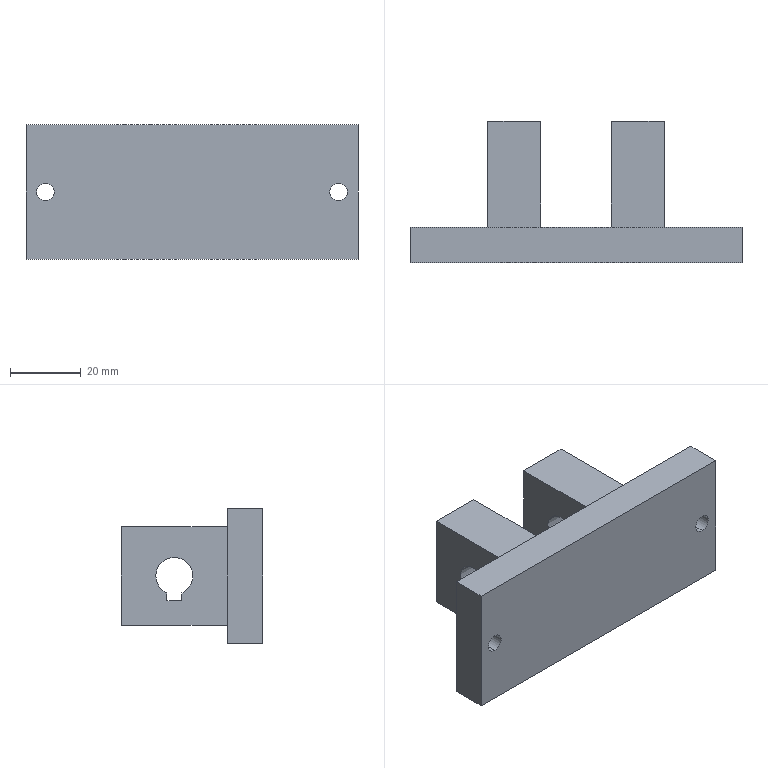Part | SolidWorks | features ICE 5, Extrusion 1, MirrorPattern 1 | 1 solid | 36 faces | box 94 x 40 x 38 mm | volume 57385 mm3 | plane 24 | cylinder 12 | commonest cylinder face diameters 5 x4 8 x4 10.5 x4
STEP:
#1=CARTESIAN_POINT('',(25.,27.1,-4.812));
#2=VERTEX_POINT('',#1);
#3=CARTESIAN_POINT('',(25.,25.,5.25));
#4=VERTEX_POINT('',#3);
#5=CARTESIAN_POINT('',(25.,25.,0.));
#6=DIRECTION('',(1.,0.,0.));
#7=DIRECTION('',(0.,0.,-1.));
#8=AXIS2_PLACEMENT_3D('',#5,#6,#7);
#9=CIRCLE('',#8,5.25);
#10=EDGE_CURVE('',#2,#4,#9,.T.);
#11=ORIENTED_EDGE('',*,*,#10,.T.);
#12=CARTESIAN_POINT('',(10.,25.,5.25));
#13=VERTEX_POINT('',#12);
#14=CARTESIAN_POINT('',(80.,25.,5.25));
#15=DIRECTION('',(-1.,0.,0.));
#16=VECTOR('',#15,1000.);
#17=LINE('',#14,#16);
#18=EDGE_CURVE('',#4,#13,#17,.T.);
#19=ORIENTED_EDGE('',*,*,#18,.T.);
#20=CARTESIAN_POINT('',(10.,27.1,-4.812));
#21=VERTEX_POINT('',#20);
#22=CARTESIAN_POINT('',(10.,25.,0.));
#23=DIRECTION('',(-1.,0.,0.));
#24=DIRECTION('',(0.,0.,1.));
#25=AXIS2_PLACEMENT_3D('',#22,#23,#24);
#26=CIRCLE('',#25,5.25);
#27=EDGE_CURVE('',#13,#21,#26,.T.);
#28=ORIENTED_EDGE('',*,*,#27,.T.);
#29=CARTESIAN_POINT('',(80.,27.1,-4.812));
#30=DIRECTION('',(-1.,0.,0.));
#31=VECTOR('',#30,1000.);
#32=LINE('',#29,#31);
#33=EDGE_CURVE('',#2,#21,#32,.T.);
#34=ORIENTED_EDGE('',*,*,#33,.F.);
#35=EDGE_LOOP('',(#11,#19,#28,#34));
#36=FACE_OUTER_BOUND('',#35,.T.);
#37=CARTESIAN_POINT('',(80.,25.,0.));
#38=DIRECTION('',(-1.,0.,0.));
#39=DIRECTION('',(0.,0.,1.));
#40=AXIS2_PLACEMENT_3D('',#37,#38,#39);
#41=CYLINDRICAL_SURFACE('',#40,5.25);
#42=ADVANCED_FACE('',(#36),#41,.F.);
#43=CARTESIAN_POINT('',(41.5,0.,2.5));
#44=VERTEX_POINT('',#43);
#45=CARTESIAN_POINT('',(41.5,0.,-2.5));
#46=VERTEX_POINT('',#45);
#47=CARTESIAN_POINT('',(41.5,0.,0.));
#48=DIRECTION('',(0.,-1.,0.));
#49=DIRECTION('',(0.,0.,1.));
#50=AXIS2_PLACEMENT_3D('',#47,#48,#49);
#51=CIRCLE('',#50,2.5);
#52=EDGE_CURVE('',#44,#46,#51,.T.);
#53=ORIENTED_EDGE('',*,*,#52,.T.);
#54=CARTESIAN_POINT('',(41.5,5.,-2.5));
#55=VERTEX_POINT('',#54);
#56=CARTESIAN_POINT('',(41.5,0.,-2.5));
#57=DIRECTION('',(0.,1.,0.));
#58=VECTOR('',#57,1000.);
#59=LINE('',#56,#58);
#60=EDGE_CURVE('',#46,#55,#59,.T.);
#61=ORIENTED_EDGE('',*,*,#60,.T.);
#62=CARTESIAN_POINT('',(41.5,5.,2.5));
#63=VERTEX_POINT('',#62);
#64=CARTESIAN_POINT('',(41.5,5.,0.));
#65=DIRECTION('',(0.,-1.,0.));
#66=DIRECTION('',(0.,0.,1.));
#67=AXIS2_PLACEMENT_3D('',#64,#65,#66);
#68=CIRCLE('',#67,2.5);
#69=EDGE_CURVE('',#63,#55,#68,.T.);
#70=ORIENTED_EDGE('',*,*,#69,.F.);
#71=CARTESIAN_POINT('',(41.5,0.,2.5));
#72=DIRECTION('',(0.,1.,0.));
#73=VECTOR('',#72,1000.);
#74=LINE('',#71,#73);
#75=EDGE_CURVE('',#44,#63,#74,.T.);
#76=ORIENTED_EDGE('',*,*,#75,.F.);
#77=EDGE_LOOP('',(#53,#61,#70,#76));
#78=FACE_OUTER_BOUND('',#77,.T.);
#79=CARTESIAN_POINT('',(41.5,0.,0.));
#80=DIRECTION('',(0.,1.,0.));
#81=DIRECTION('',(0.,0.,1.));
#82=AXIS2_PLACEMENT_3D('',#79,#80,#81);
#83=CYLINDRICAL_SURFACE('',#82,2.5);
#84=ADVANCED_FACE('',(#78),#83,.F.);
#85=CARTESIAN_POINT('',(41.5,5.,4.));
#86=VERTEX_POINT('',#85);
#87=CARTESIAN_POINT('',(41.5,5.,-4.));
#88=VERTEX_POINT('',#87);
#89=CARTESIAN_POINT('',(41.5,5.,0.));
#90=DIRECTION('',(0.,-1.,0.));
#91=DIRECTION('',(0.,0.,1.));
#92=AXIS2_PLACEMENT_3D('',#89,#90,#91);
#93=CIRCLE('',#92,4.);
#94=EDGE_CURVE('',#86,#88,#93,.T.);
#95=ORIENTED_EDGE('',*,*,#94,.T.);
#96=CARTESIAN_POINT('',(41.5,10.,-4.));
#97=VERTEX_POINT('',#96);
#98=CARTESIAN_POINT('',(41.5,5.,-4.));
#99=DIRECTION('',(0.,1.,0.));
#100=VECTOR('',#99,1000.);
#101=LINE('',#98,#100);
#102=EDGE_CURVE('',#88,#97,#101,.T.);
#103=ORIENTED_EDGE('',*,*,#102,.T.);
#104=CARTESIAN_POINT('',(41.5,10.,4.));
#105=VERTEX_POINT('',#104);
#106=CARTESIAN_POINT('',(41.5,10.,0.));
#107=DIRECTION('',(0.,-1.,0.));
#108=DIRECTION('',(0.,0.,1.));
#109=AXIS2_PLACEMENT_3D('',#106,#107,#108);
#110=CIRCLE('',#109,4.);
#111=EDGE_CURVE('',#105,#97,#110,.T.);
#112=ORIENTED_EDGE('',*,*,#111,.F.);
#113=CARTESIAN_POINT('',(41.5,5.,4.));
#114=DIRECTION('',(0.,1.,0.));
#115=VECTOR('',#114,1000.);
#116=LINE('',#113,#115);
#117=EDGE_CURVE('',#86,#105,#116,.T.);
#118=ORIENTED_EDGE('',*,*,#117,.F.);
#119=EDGE_LOOP('',(#95,#103,#112,#118));
#120=FACE_OUTER_BOUND('',#119,.T.);
#121=CARTESIAN_POINT('',(41.5,5.,0.));
#122=DIRECTION('',(0.,1.,0.));
#123=DIRECTION('',(0.,0.,1.));
#124=AXIS2_PLACEMENT_3D('',#121,#122,#123);
#125=CYLINDRICAL_SURFACE('',#124,4.);
#126=ADVANCED_FACE('',(#120),#125,.F.);
#127=CARTESIAN_POINT('',(-10.,25.,5.25));
#128=VERTEX_POINT('',#127);
#129=CARTESIAN_POINT('',(-10.,27.1,-4.812));
#130=VERTEX_POINT('',#129);
#131=CARTESIAN_POINT('',(-10.,25.,0.));
#132=DIRECTION('',(-1.,0.,0.));
#133=DIRECTION('',(0.,0.,1.));
#134=AXIS2_PLACEMENT_3D('',#131,#132,#133);
#135=CIRCLE('',#134,5.25);
#136=EDGE_CURVE('',#128,#130,#135,.T.);
#137=ORIENTED_EDGE('',*,*,#136,.F.);
#138=CARTESIAN_POINT('',(-25.,25.,5.25));
#139=VERTEX_POINT('',#138);
#140=CARTESIAN_POINT('',(84.,25.,5.25));
#141=DIRECTION('',(-1.,0.,0.));
#142=VECTOR('',#141,1000.);
#143=LINE('',#140,#142);
#144=EDGE_CURVE('',#128,#139,#143,.T.);
#145=ORIENTED_EDGE('',*,*,#144,.T.);
#146=CARTESIAN_POINT('',(-25.,27.1,-4.812));
#147=VERTEX_POINT('',#146);
#148=CARTESIAN_POINT('',(-25.,25.,0.));
#149=DIRECTION('',(-1.,0.,0.));
#150=DIRECTION('',(0.,0.,1.));
#151=AXIS2_PLACEMENT_3D('',#148,#149,#150);
#152=CIRCLE('',#151,5.25);
#153=EDGE_CURVE('',#139,#147,#152,.T.);
#154=ORIENTED_EDGE('',*,*,#153,.T.);
#155=CARTESIAN_POINT('',(84.,27.1,-4.812));
#156=DIRECTION('',(-1.,0.,0.));
#157=VECTOR('',#156,1000.);
#158=LINE('',#155,#157);
#159=EDGE_CURVE('',#130,#147,#158,.T.);
#160=ORIENTED_EDGE('',*,*,#159,.F.);
#161=EDGE_LOOP('',(#137,#145,#154,#160));
#162=FACE_OUTER_BOUND('',#161,.T.);
#163=CARTESIAN_POINT('',(84.,25.,0.));
#164=DIRECTION('',(-1.,0.,0.));
#165=DIRECTION('',(0.,0.,1.));
#166=AXIS2_PLACEMENT_3D('',#163,#164,#165);
#167=CYLINDRICAL_SURFACE('',#166,5.25);
#168=ADVANCED_FACE('',(#162),#167,.F.);
#169=CARTESIAN_POINT('',(-41.5,0.,-2.5));
#170=VERTEX_POINT('',#169);
#171=CARTESIAN_POINT('',(-41.5,0.,2.5));
#172=VERTEX_POINT('',#171);
#173=CARTESIAN_POINT('',(-41.5,0.,0.));
#174=DIRECTION('',(0.,1.,0.));
#175=DIRECTION('',(0.,0.,1.));
#176=AXIS2_PLACEMENT_3D('',#173,#174,#175);
#177=CIRCLE('',#176,2.5);
#178=EDGE_CURVE('',#170,#172,#177,.T.);
#179=ORIENTED_EDGE('',*,*,#178,.F.);
#180=CARTESIAN_POINT('',(-41.5,5.,-2.5));
#181=VERTEX_POINT('',#180);
#182=CARTESIAN_POINT('',(-41.5,0.,-2.5));
#183=DIRECTION('',(0.,1.,0.));
#184=VECTOR('',#183,1000.);
#185=LINE('',#182,#184);
#186=EDGE_CURVE('',#170,#181,#185,.T.);
#187=ORIENTED_EDGE('',*,*,#186,.T.);
#188=CARTESIAN_POINT('',(-41.5,5.,2.5));
#189=VERTEX_POINT('',#188);
#190=CARTESIAN_POINT('',(-41.5,5.,0.));
#191=DIRECTION('',(0.,1.,0.));
#192=DIRECTION('',(0.,0.,1.));
#193=AXIS2_PLACEMENT_3D('',#190,#191,#192);
#194=CIRCLE('',#193,2.5);
#195=EDGE_CURVE('',#181,#189,#194,.T.);
#196=ORIENTED_EDGE('',*,*,#195,.T.);
#197=CARTESIAN_POINT('',(-41.5,0.,2.5));
#198=DIRECTION('',(0.,1.,0.));
#199=VECTOR('',#198,1000.);
#200=LINE('',#197,#199);
#201=EDGE_CURVE('',#172,#189,#200,.T.);
#202=ORIENTED_EDGE('',*,*,#201,.F.);
#203=EDGE_LOOP('',(#179,#187,#196,#202));
#204=FACE_OUTER_BOUND('',#203,.T.);
#205=CARTESIAN_POINT('',(-41.5,0.,0.));
#206=DIRECTION('',(0.,1.,0.));
#207=DIRECTION('',(0.,0.,1.));
#208=AXIS2_PLACEMENT_3D('',#205,#206,#207);
#209=CYLINDRICAL_SURFACE('',#208,2.5);
#210=ADVANCED_FACE('',(#204),#209,.F.);
#211=CARTESIAN_POINT('',(-41.5,5.,-4.));
#212=VERTEX_POINT('',#211);
#213=CARTESIAN_POINT('',(-41.5,5.,4.));
#214=VERTEX_POINT('',#213);
#215=CARTESIAN_POINT('',(-41.5,5.,0.));
#216=DIRECTION('',(0.,1.,0.));
#217=DIRECTION('',(0.,0.,1.));
#218=AXIS2_PLACEMENT_3D('',#215,#216,#217);
#219=CIRCLE('',#218,4.);
#220=EDGE_CURVE('',#212,#214,#219,.T.);
#221=ORIENTED_EDGE('',*,*,#220,.F.);
#222=CARTESIAN_POINT('',(-41.5,10.,-4.));
#223=VERTEX_POINT('',#222);
#224=CARTESIAN_POINT('',(-41.5,5.,-4.));
#225=DIRECTION('',(0.,1.,0.));
#226=VECTOR('',#225,1000.);
#227=LINE('',#224,#226);
#228=EDGE_CURVE('',#212,#223,#227,.T.);
#229=ORIENTED_EDGE('',*,*,#228,.T.);
#230=CARTESIAN_POINT('',(-41.5,10.,4.));
#231=VERTEX_POINT('',#230);
#232=CARTESIAN_POINT('',(-41.5,10.,0.));
#233=DIRECTION('',(0.,1.,0.));
#234=DIRECTION('',(0.,0.,1.));
#235=AXIS2_PLACEMENT_3D('',#232,#233,#234);
#236=CIRCLE('',#235,4.);
#237=EDGE_CURVE('',#223,#231,#236,.T.);
#238=ORIENTED_EDGE('',*,*,#237,.T.);
#239=CARTESIAN_POINT('',(-41.5,5.,4.));
#240=DIRECTION('',(0.,1.,0.));
#241=VECTOR('',#240,1000.);
#242=LINE('',#239,#241);
#243=EDGE_CURVE('',#214,#231,#242,.T.);
#244=ORIENTED_EDGE('',*,*,#243,.F.);
#245=EDGE_LOOP('',(#221,#229,#238,#244));
#246=FACE_OUTER_BOUND('',#245,.T.);
#247=CARTESIAN_POINT('',(-41.5,5.,0.));
#248=DIRECTION('',(0.,1.,0.));
#249=DIRECTION('',(0.,0.,1.));
#250=AXIS2_PLACEMENT_3D('',#247,#248,#249);
#251=CYLINDRICAL_SURFACE('',#250,4.);
#252=ADVANCED_FACE('',(#246),#251,.F.);
#253=CARTESIAN_POINT('',(-10.,10.,-14.));
#254=VERTEX_POINT('',#253);
#255=CARTESIAN_POINT('',(-10.,10.,14.));
#256=VERTEX_POINT('',#255);
#257=CARTESIAN_POINT('',(-10.,10.,14.));
#258=DIRECTION('',(0.,0.,1.));
#259=VECTOR('',#258,1000.);
#260=LINE('',#257,#259);
#261=EDGE_CURVE('',#254,#256,#260,.T.);
#262=ORIENTED_EDGE('',*,*,#261,.T.);
#263=CARTESIAN_POINT('',(-25.,10.,14.));
#264=VERTEX_POINT('',#263);
#265=CARTESIAN_POINT('',(-10.,10.,14.));
#266=DIRECTION('',(-1.,0.,0.));
#267=VECTOR('',#266,1000.);
#268=LINE('',#265,#267);
#269=EDGE_CURVE('',#256,#264,#268,.T.);
#270=ORIENTED_EDGE('',*,*,#269,.T.);
#271=CARTESIAN_POINT('',(-25.,10.,-14.));
#272=VERTEX_POINT('',#271);
#273=CARTESIAN_POINT('',(-25.,10.,14.));
#274=DIRECTION('',(0.,0.,1.));
#275=VECTOR('',#274,1000.);
#276=LINE('',#273,#275);
#277=EDGE_CURVE('',#272,#264,#276,.T.);
#278=ORIENTED_EDGE('',*,*,#277,.F.);
#279=CARTESIAN_POINT('',(-10.,10.,-14.));
#280=DIRECTION('',(-1.,0.,0.));
#281=VECTOR('',#280,1000.);
#282=LINE('',#279,#281);
#283=EDGE_CURVE('',#254,#272,#282,.T.);
#284=ORIENTED_EDGE('',*,*,#283,.F.);
#285=EDGE_LOOP('',(#262,#270,#278,#284));
#286=FACE_BOUND('',#285,.T.);
#287=CARTESIAN_POINT('',(-41.5,10.,0.));
#288=DIRECTION('',(0.,1.,0.));
#289=DIRECTION('',(0.,0.,1.));
#290=AXIS2_PLACEMENT_3D('',#287,#288,#289);
#291=CIRCLE('',#290,4.);
#292=EDGE_CURVE('',#231,#223,#291,.T.);
#293=ORIENTED_EDGE('',*,*,#292,.F.);
#294=ORIENTED_EDGE('',*,*,#237,.F.);
#295=EDGE_LOOP('',(#293,#294));
#296=FACE_BOUND('',#295,.T.);
#297=CARTESIAN_POINT('',(47.,10.,19.));
#298=VERTEX_POINT('',#297);
#299=CARTESIAN_POINT('',(47.,10.,-19.));
#300=VERTEX_POINT('',#299);
#301=CARTESIAN_POINT('',(47.,10.,19.));
#302=DIRECTION('',(0.,0.,-1.));
#303=VECTOR('',#302,1000.);
#304=LINE('',#301,#303);
#305=EDGE_CURVE('',#298,#300,#304,.T.);
#306=ORIENTED_EDGE('',*,*,#305,.T.);
#307=CARTESIAN_POINT('',(-47.,10.,-19.));
#308=VERTEX_POINT('',#307);
#309=CARTESIAN_POINT('',(-47.,10.,-19.));
#310=DIRECTION('',(-1.,0.,0.));
#311=VECTOR('',#310,1000.);
#312=LINE('',#309,#311);
#313=EDGE_CURVE('',#300,#308,#312,.T.);
#314=ORIENTED_EDGE('',*,*,#313,.T.);
#315=CARTESIAN_POINT('',(-47.,10.,19.));
#316=VERTEX_POINT('',#315);
#317=CARTESIAN_POINT('',(-47.,10.,19.));
#318=DIRECTION('',(0.,0.,1.));
#319=VECTOR('',#318,1000.);
#320=LINE('',#317,#319);
#321=EDGE_CURVE('',#308,#316,#320,.T.);
#322=ORIENTED_EDGE('',*,*,#321,.T.);
#323=CARTESIAN_POINT('',(-47.,10.,19.));
#324=DIRECTION('',(1.,0.,0.));
#325=VECTOR('',#324,1000.);
#326=LINE('',#323,#325);
#327=EDGE_CURVE('',#316,#298,#326,.T.);
#328=ORIENTED_EDGE('',*,*,#327,.T.);
#329=EDGE_LOOP('',(#306,#314,#322,#328));
#330=FACE_OUTER_BOUND('',#329,.T.);
#331=ORIENTED_EDGE('',*,*,#111,.T.);
#332=CARTESIAN_POINT('',(41.5,10.,0.));
#333=DIRECTION('',(0.,-1.,0.));
#334=DIRECTION('',(0.,0.,1.));
#335=AXIS2_PLACEMENT_3D('',#332,#333,#334);
#336=CIRCLE('',#335,4.);
#337=EDGE_CURVE('',#97,#105,#336,.T.);
#338=ORIENTED_EDGE('',*,*,#337,.T.);
#339=EDGE_LOOP('',(#331,#338));
#340=FACE_BOUND('',#339,.T.);
#341=CARTESIAN_POINT('',(10.,10.,-14.));
#342=VERTEX_POINT('',#341);
#343=CARTESIAN_POINT('',(10.,10.,14.));
#344=VERTEX_POINT('',#343);
#345=CARTESIAN_POINT('',(10.,10.,14.));
#346=DIRECTION('',(0.,0.,1.));
#347=VECTOR('',#346,1000.);
#348=LINE('',#345,#347);
#349=EDGE_CURVE('',#342,#344,#348,.T.);
#350=ORIENTED_EDGE('',*,*,#349,.F.);
#351=CARTESIAN_POINT('',(25.,10.,-14.));
#352=VERTEX_POINT('',#351);
#353=CARTESIAN_POINT('',(10.,10.,-14.));
#354=DIRECTION('',(1.,0.,0.));
#355=VECTOR('',#354,1000.);
#356=LINE('',#353,#355);
#357=EDGE_CURVE('',#342,#352,#356,.T.);
#358=ORIENTED_EDGE('',*,*,#357,.T.);
#359=CARTESIAN_POINT('',(25.,10.,14.));
#360=VERTEX_POINT('',#359);
#361=CARTESIAN_POINT('',(25.,10.,14.));
#362=DIRECTION('',(0.,0.,1.));
#363=VECTOR('',#362,1000.);
#364=LINE('',#361,#363);
#365=EDGE_CURVE('',#352,#360,#364,.T.);
#366=ORIENTED_EDGE('',*,*,#365,.T.);
#367=CARTESIAN_POINT('',(10.,10.,14.));
#368=DIRECTION('',(1.,0.,0.));
#369=VECTOR('',#368,1000.);
#370=LINE('',#367,#369);
#371=EDGE_CURVE('',#344,#360,#370,.T.);
#372=ORIENTED_EDGE('',*,*,#371,.F.);
#373=EDGE_LOOP('',(#350,#358,#366,#372));
#374=FACE_BOUND('',#373,.T.);
#375=CARTESIAN_POINT('',(0.,10.,0.));
#376=DIRECTION('',(0.,-1.,0.));
#377=DIRECTION('',(0.,0.,-1.));
#378=AXIS2_PLACEMENT_3D('',#375,#376,#377);
#379=PLANE('',#378);
#380=ADVANCED_FACE('',(#286,#296,#330,#340,#374),#379,.F.);
#381=CARTESIAN_POINT('',(47.,0.,19.));
#382=VERTEX_POINT('',#381);
#383=CARTESIAN_POINT('',(47.,0.,-19.));
#384=VERTEX_POINT('',#383);
#385=CARTESIAN_POINT('',(47.,0.,19.));
#386=DIRECTION('',(0.,0.,-1.));
#387=VECTOR('',#386,1000.);
#388=LINE('',#385,#387);
#389=EDGE_CURVE('',#382,#384,#388,.T.);
#390=ORIENTED_EDGE('',*,*,#389,.T.);
#391=CARTESIAN_POINT('',(47.,10.,-19.));
#392=DIRECTION('',(0.,-1.,0.));
#393=VECTOR('',#392,1000.);
#394=LINE('',#391,#393);
#395=EDGE_CURVE('',#300,#384,#394,.T.);
#396=ORIENTED_EDGE('',*,*,#395,.F.);
#397=ORIENTED_EDGE('',*,*,#305,.F.);
#398=CARTESIAN_POINT('',(47.,10.,19.));
#399=DIRECTION('',(0.,-1.,0.));
#400=VECTOR('',#399,1000.);
#401=LINE('',#398,#400);
#402=EDGE_CURVE('',#298,#382,#401,.T.);
#403=ORIENTED_EDGE('',*,*,#402,.T.);
#404=EDGE_LOOP('',(#390,#396,#397,#403));
#405=FACE_OUTER_BOUND('',#404,.T.);
#406=CARTESIAN_POINT('',(47.,10.,19.));
#407=DIRECTION('',(-1.,0.,0.));
#408=DIRECTION('',(0.,0.,1.));
#409=AXIS2_PLACEMENT_3D('',#406,#407,#408);
#410=PLANE('',#409);
#411=ADVANCED_FACE('',(#405),#410,.F.);
#412=CARTESIAN_POINT('',(-47.,0.,-19.));
#413=VERTEX_POINT('',#412);
#414=CARTESIAN_POINT('',(-47.,0.,-19.));
#415=DIRECTION('',(-1.,0.,0.));
#416=VECTOR('',#415,1000.);
#417=LINE('',#414,#416);
#418=EDGE_CURVE('',#384,#413,#417,.T.);
#419=ORIENTED_EDGE('',*,*,#418,.T.);
#420=CARTESIAN_POINT('',(-47.,10.,-19.));
#421=DIRECTION('',(0.,-1.,0.));
#422=VECTOR('',#421,1000.);
#423=LINE('',#420,#422);
#424=EDGE_CURVE('',#308,#413,#423,.T.);
#425=ORIENTED_EDGE('',*,*,#424,.F.);
#426=ORIENTED_EDGE('',*,*,#313,.F.);
#427=ORIENTED_EDGE('',*,*,#395,.T.);
#428=EDGE_LOOP('',(#419,#425,#426,#427));
#429=FACE_OUTER_BOUND('',#428,.T.);
#430=CARTESIAN_POINT('',(-47.,10.,-19.));
#431=DIRECTION('',(0.,0.,1.));
#432=DIRECTION('',(1.,0.,0.));
#433=AXIS2_PLACEMENT_3D('',#430,#431,#432);
#434=PLANE('',#433);
#435=ADVANCED_FACE('',(#429),#434,.F.);
#436=CARTESIAN_POINT('',(-47.,0.,19.));
#437=VERTEX_POINT('',#436);
#438=CARTESIAN_POINT('',(-47.,0.,19.));
#439=DIRECTION('',(0.,0.,1.));
#440=VECTOR('',#439,1000.);
#441=LINE('',#438,#440);
#442=EDGE_CURVE('',#413,#437,#441,.T.);
#443=ORIENTED_EDGE('',*,*,#442,.T.);
#444=CARTESIAN_POINT('',(-47.,10.,19.));
#445=DIRECTION('',(0.,-1.,0.));
#446=VECTOR('',#445,1000.);
#447=LINE('',#444,#446);
#448=EDGE_CURVE('',#316,#437,#447,.T.);
#449=ORIENTED_EDGE('',*,*,#448,.F.);
#450=ORIENTED_EDGE('',*,*,#321,.F.);
#451=ORIENTED_EDGE('',*,*,#424,.T.);
#452=EDGE_LOOP('',(#443,#449,#450,#451));
#453=FACE_OUTER_BOUND('',#452,.T.);
#454=CARTESIAN_POINT('',(-47.,10.,19.));
#455=DIRECTION('',(1.,0.,0.));
#456=DIRECTION('',(0.,0.,-1.));
#457=AXIS2_PLACEMENT_3D('',#454,#455,#456);
#458=PLANE('',#457);
#459=ADVANCED_FACE('',(#453),#458,.F.);
#460=CARTESIAN_POINT('',(-47.,0.,19.));
#461=DIRECTION('',(1.,0.,0.));
#462=VECTOR('',#461,1000.);
#463=LINE('',#460,#462);
#464=EDGE_CURVE('',#437,#382,#463,.T.);
#465=ORIENTED_EDGE('',*,*,#464,.T.);
#466=ORIENTED_EDGE('',*,*,#402,.F.);
#467=ORIENTED_EDGE('',*,*,#327,.F.);
#468=ORIENTED_EDGE('',*,*,#448,.T.);
#469=EDGE_LOOP('',(#465,#466,#467,#468));
#470=FACE_OUTER_BOUND('',#469,.T.);
#471=CARTESIAN_POINT('',(-47.,10.,19.));
#472=DIRECTION('',(0.,0.,-1.));
#473=DIRECTION('',(-1.,0.,0.));
#474=AXIS2_PLACEMENT_3D('',#471,#472,#473);
#475=PLANE('',#474);
#476=ADVANCED_FACE('',(#470),#475,.F.);
#477=ORIENTED_EDGE('',*,*,#52,.F.);
#478=CARTESIAN_POINT('',(41.5,0.,0.));
#479=DIRECTION('',(0.,-1.,0.));
#480=DIRECTION('',(0.,0.,1.));
#481=AXIS2_PLACEMENT_3D('',#478,#479,#480);
#482=CIRCLE('',#481,2.5);
#483=EDGE_CURVE('',#46,#44,#482,.T.);
#484=ORIENTED_EDGE('',*,*,#483,.F.);
#485=EDGE_LOOP('',(#477,#484));
#486=FACE_BOUND('',#485,.T.);
#487=CARTESIAN_POINT('',(-41.5,0.,0.));
#488=DIRECTION('',(0.,1.,0.));
#489=DIRECTION('',(0.,0.,1.));
#490=AXIS2_PLACEMENT_3D('',#487,#488,#489);
#491=CIRCLE('',#490,2.5);
#492=EDGE_CURVE('',#172,#170,#491,.T.);
#493=ORIENTED_EDGE('',*,*,#492,.T.);
#494=ORIENTED_EDGE('',*,*,#178,.T.);
#495=EDGE_LOOP('',(#493,#494));
#496=FACE_BOUND('',#495,.T.);
#497=ORIENTED_EDGE('',*,*,#389,.F.);
#498=ORIENTED_EDGE('',*,*,#464,.F.);
#499=ORIENTED_EDGE('',*,*,#442,.F.);
#500=ORIENTED_EDGE('',*,*,#418,.F.);
#501=EDGE_LOOP('',(#497,#498,#499,#500));
#502=FACE_OUTER_BOUND('',#501,.T.);
#503=CARTESIAN_POINT('',(0.,0.,0.));
#504=DIRECTION('',(0.,-1.,0.));
#505=DIRECTION('',(0.,0.,-1.));
#506=AXIS2_PLACEMENT_3D('',#503,#504,#505);
#507=PLANE('',#506);
#508=ADVANCED_FACE('',(#486,#496,#502),#507,.T.);
#509=ORIENTED_EDGE('',*,*,#228,.F.);
#510=CARTESIAN_POINT('',(-41.5,5.,0.));
#511=DIRECTION('',(0.,1.,0.));
#512=DIRECTION('',(0.,0.,1.));
#513=AXIS2_PLACEMENT_3D('',#510,#511,#512);
#514=CIRCLE('',#513,4.);
#515=EDGE_CURVE('',#214,#212,#514,.T.);
#516=ORIENTED_EDGE('',*,*,#515,.F.);
#517=ORIENTED_EDGE('',*,*,#243,.T.);
#518=ORIENTED_EDGE('',*,*,#292,.T.);
#519=EDGE_LOOP('',(#509,#516,#517,#518));
#520=FACE_OUTER_BOUND('',#519,.T.);
#521=CARTESIAN_POINT('',(-41.5,5.,0.));
#522=DIRECTION('',(0.,1.,0.));
#523=DIRECTION('',(0.,0.,1.));
#524=AXIS2_PLACEMENT_3D('',#521,#522,#523);
#525=CYLINDRICAL_SURFACE('',#524,4.);
#526=ADVANCED_FACE('',(#520),#525,.F.);
#527=CARTESIAN_POINT('',(-41.5,5.,0.));
#528=DIRECTION('',(0.,1.,0.));
#529=DIRECTION('',(0.,0.,1.));
#530=AXIS2_PLACEMENT_3D('',#527,#528,#529);
#531=CIRCLE('',#530,2.5);
#532=EDGE_CURVE('',#189,#181,#531,.T.);
#533=ORIENTED_EDGE('',*,*,#532,.F.);
#534=ORIENTED_EDGE('',*,*,#195,.F.);
#535=EDGE_LOOP('',(#533,#534));
#536=FACE_BOUND('',#535,.T.);
#537=ORIENTED_EDGE('',*,*,#515,.T.);
#538=ORIENTED_EDGE('',*,*,#220,.T.);
#539=EDGE_LOOP('',(#537,#538));
#540=FACE_OUTER_BOUND('',#539,.T.);
#541=CARTESIAN_POINT('',(-41.5,5.,0.));
#542=DIRECTION('',(0.,1.,0.));
#543=DIRECTION('',(0.,0.,1.));
#544=AXIS2_PLACEMENT_3D('',#541,#542,#543);
#545=PLANE('',#544);
#546=ADVANCED_FACE('',(#536,#540),#545,.T.);
#547=ORIENTED_EDGE('',*,*,#186,.F.);
#548=ORIENTED_EDGE('',*,*,#492,.F.);
#549=ORIENTED_EDGE('',*,*,#201,.T.);
#550=ORIENTED_EDGE('',*,*,#532,.T.);
#551=EDGE_LOOP('',(#547,#548,#549,#550));
#552=FACE_OUTER_BOUND('',#551,.T.);
#553=CARTESIAN_POINT('',(-41.5,0.,0.));
#554=DIRECTION('',(0.,1.,0.));
#555=DIRECTION('',(0.,0.,1.));
#556=AXIS2_PLACEMENT_3D('',#553,#554,#555);
#557=CYLINDRICAL_SURFACE('',#556,2.5);
#558=ADVANCED_FACE('',(#552),#557,.F.);
#559=CARTESIAN_POINT('',(-25.,40.,14.));
#560=VERTEX_POINT('',#559);
#561=CARTESIAN_POINT('',(-25.,10.,14.));
#562=DIRECTION('',(0.,1.,0.));
#563=VECTOR('',#562,1000.);
#564=LINE('',#561,#563);
#565=EDGE_CURVE('',#264,#560,#564,.T.);
#566=ORIENTED_EDGE('',*,*,#565,.F.);
#567=ORIENTED_EDGE('',*,*,#269,.F.);
#568=CARTESIAN_POINT('',(-10.,40.,14.));
#569=VERTEX_POINT('',#568);
#570=CARTESIAN_POINT('',(-10.,10.,14.));
#571=DIRECTION('',(0.,1.,0.));
#572=VECTOR('',#571,1000.);
#573=LINE('',#570,#572);
#574=EDGE_CURVE('',#256,#569,#573,.T.);
#575=ORIENTED_EDGE('',*,*,#574,.T.);
#576=CARTESIAN_POINT('',(-10.,40.,14.));
#577=DIRECTION('',(-1.,0.,0.));
#578=VECTOR('',#577,1000.);
#579=LINE('',#576,#578);
#580=EDGE_CURVE('',#569,#560,#579,.T.);
#581=ORIENTED_EDGE('',*,*,#580,.T.);
#582=EDGE_LOOP('',(#566,#567,#575,#581));
#583=FACE_OUTER_BOUND('',#582,.T.);
#584=CARTESIAN_POINT('',(-10.,10.,14.));
#585=DIRECTION('',(0.,0.,1.));
#586=DIRECTION('',(0.,-1.,0.));
#587=AXIS2_PLACEMENT_3D('',#584,#585,#586);
#588=PLANE('',#587);
#589=ADVANCED_FACE('',(#583),#588,.T.);
#590=CARTESIAN_POINT('',(-25.,40.,-14.));
#591=VERTEX_POINT('',#590);
#592=CARTESIAN_POINT('',(-25.,10.,-14.));
#593=DIRECTION('',(0.,-1.,0.));
#594=VECTOR('',#593,1000.);
#595=LINE('',#592,#594);
#596=EDGE_CURVE('',#591,#272,#595,.T.);
#597=ORIENTED_EDGE('',*,*,#596,.F.);
#598=CARTESIAN_POINT('',(-10.,40.,-14.));
#599=VERTEX_POINT('',#598);
#600=CARTESIAN_POINT('',(-10.,40.,-14.));
#601=DIRECTION('',(-1.,0.,0.));
#602=VECTOR('',#601,1000.);
#603=LINE('',#600,#602);
#604=EDGE_CURVE('',#599,#591,#603,.T.);
#605=ORIENTED_EDGE('',*,*,#604,.F.);
#606=CARTESIAN_POINT('',(-10.,10.,-14.));
#607=DIRECTION('',(0.,-1.,0.));
#608=VECTOR('',#607,1000.);
#609=LINE('',#606,#608);
#610=EDGE_CURVE('',#599,#254,#609,.T.);
#611=ORIENTED_EDGE('',*,*,#610,.T.);
#612=ORIENTED_EDGE('',*,*,#283,.T.);
#613=EDGE_LOOP('',(#597,#605,#611,#612));
#614=FACE_OUTER_BOUND('',#613,.T.);
#615=CARTESIAN_POINT('',(-10.,10.,-14.));
#616=DIRECTION('',(0.,0.,-1.));
#617=DIRECTION('',(-1.,0.,0.));
#618=AXIS2_PLACEMENT_3D('',#615,#616,#617);
#619=PLANE('',#618);
#620=ADVANCED_FACE('',(#614),#619,.T.);
#621=CARTESIAN_POINT('',(-25.,40.,14.));
#622=DIRECTION('',(0.,0.,-1.));
#623=VECTOR('',#622,1000.);
#624=LINE('',#621,#623);
#625=EDGE_CURVE('',#560,#591,#624,.T.);
#626=ORIENTED_EDGE('',*,*,#625,.F.);
#627=ORIENTED_EDGE('',*,*,#580,.F.);
#628=CARTESIAN_POINT('',(-10.,40.,14.));
#629=DIRECTION('',(0.,0.,-1.));
#630=VECTOR('',#629,1000.);
#631=LINE('',#628,#630);
#632=EDGE_CURVE('',#569,#599,#631,.T.);
#633=ORIENTED_EDGE('',*,*,#632,.T.);
#634=ORIENTED_EDGE('',*,*,#604,.T.);
#635=EDGE_LOOP('',(#626,#627,#633,#634));
#636=FACE_OUTER_BOUND('',#635,.T.);
#637=CARTESIAN_POINT('',(-10.,40.,14.));
#638=DIRECTION('',(0.,1.,0.));
#639=DIRECTION('',(0.,0.,1.));
#640=AXIS2_PLACEMENT_3D('',#637,#638,#639);
#641=PLANE('',#640);
#642=ADVANCED_FACE('',(#636),#641,.T.);
#643=CARTESIAN_POINT('',(-10.,27.1,-7.));
#644=VERTEX_POINT('',#643);
#645=CARTESIAN_POINT('',(-10.,27.1,0.));
#646=DIRECTION('',(0.,0.,1.));
#647=VECTOR('',#646,1000.);
#648=LINE('',#645,#647);
#649=EDGE_CURVE('',#644,#130,#648,.T.);
#650=ORIENTED_EDGE('',*,*,#649,.F.);
#651=CARTESIAN_POINT('',(-10.,22.9,-7.));
#652=VERTEX_POINT('',#651);
#653=CARTESIAN_POINT('',(-10.,0.,-7.));
#654=DIRECTION('',(0.,-1.,0.));
#655=VECTOR('',#654,1000.);
#656=LINE('',#653,#655);
#657=EDGE_CURVE('',#644,#652,#656,.T.);
#658=ORIENTED_EDGE('',*,*,#657,.T.);
#659=CARTESIAN_POINT('',(-10.,22.9,-4.812));
#660=VERTEX_POINT('',#659);
#661=CARTESIAN_POINT('',(-10.,22.9,0.));
#662=DIRECTION('',(0.,0.,1.));
#663=VECTOR('',#662,1000.);
#664=LINE('',#661,#663);
#665=EDGE_CURVE('',#652,#660,#664,.T.);
#666=ORIENTED_EDGE('',*,*,#665,.T.);
#667=CARTESIAN_POINT('',(-10.,25.,0.));
#668=DIRECTION('',(-1.,0.,0.));
#669=DIRECTION('',(0.,0.,1.));
#670=AXIS2_PLACEMENT_3D('',#667,#668,#669);
#671=CIRCLE('',#670,5.25);
#672=EDGE_CURVE('',#660,#128,#671,.T.);
#673=ORIENTED_EDGE('',*,*,#672,.T.);
#674=ORIENTED_EDGE('',*,*,#136,.T.);
#675=EDGE_LOOP('',(#650,#658,#666,#673,#674));
#676=FACE_BOUND('',#675,.T.);
#677=ORIENTED_EDGE('',*,*,#574,.F.);
#678=ORIENTED_EDGE('',*,*,#261,.F.);
#679=ORIENTED_EDGE('',*,*,#610,.F.);
#680=ORIENTED_EDGE('',*,*,#632,.F.);
#681=EDGE_LOOP('',(#677,#678,#679,#680));
#682=FACE_OUTER_BOUND('',#681,.T.);
#683=CARTESIAN_POINT('',(-10.,0.,0.));
#684=DIRECTION('',(-1.,0.,0.));
#685=DIRECTION('',(0.,0.,1.));
#686=AXIS2_PLACEMENT_3D('',#683,#684,#685);
#687=PLANE('',#686);
#688=ADVANCED_FACE('',(#676,#682),#687,.F.);
#689=CARTESIAN_POINT('',(-25.,27.1,-7.));
#690=VERTEX_POINT('',#689);
#691=CARTESIAN_POINT('',(-25.,22.9,-7.));
#692=VERTEX_POINT('',#691);
#693=CARTESIAN_POINT('',(-25.,27.1,-7.));
#694=DIRECTION('',(0.,-1.,0.));
#695=VECTOR('',#694,1000.);
#696=LINE('',#693,#695);
#697=EDGE_CURVE('',#690,#692,#696,.T.);
#698=ORIENTED_EDGE('',*,*,#697,.F.);
#699=CARTESIAN_POINT('',(-25.,27.1,-7.));
#700=DIRECTION('',(0.,0.,1.));
#701=VECTOR('',#700,1000.);
#702=LINE('',#699,#701);
#703=EDGE_CURVE('',#690,#147,#702,.T.);
#704=ORIENTED_EDGE('',*,*,#703,.T.);
#705=ORIENTED_EDGE('',*,*,#153,.F.);
#706=CARTESIAN_POINT('',(-25.,22.9,-4.812));
#707=VERTEX_POINT('',#706);
#708=CARTESIAN_POINT('',(-25.,25.,0.));
#709=DIRECTION('',(-1.,0.,0.));
#710=DIRECTION('',(0.,0.,1.));
#711=AXIS2_PLACEMENT_3D('',#708,#709,#710);
#712=CIRCLE('',#711,5.25);
#713=EDGE_CURVE('',#707,#139,#712,.T.);
#714=ORIENTED_EDGE('',*,*,#713,.F.);
#715=CARTESIAN_POINT('',(-25.,22.9,-7.));
#716=DIRECTION('',(0.,0.,1.));
#717=VECTOR('',#716,1000.);
#718=LINE('',#715,#717);
#719=EDGE_CURVE('',#692,#707,#718,.T.);
#720=ORIENTED_EDGE('',*,*,#719,.F.);
#721=EDGE_LOOP('',(#698,#704,#705,#714,#720));
#722=FACE_BOUND('',#721,.T.);
#723=ORIENTED_EDGE('',*,*,#565,.T.);
#724=ORIENTED_EDGE('',*,*,#625,.T.);
#725=ORIENTED_EDGE('',*,*,#596,.T.);
#726=ORIENTED_EDGE('',*,*,#277,.T.);
#727=EDGE_LOOP('',(#723,#724,#725,#726));
#728=FACE_OUTER_BOUND('',#727,.T.);
#729=CARTESIAN_POINT('',(-25.,0.,0.));
#730=DIRECTION('',(-1.,0.,0.));
#731=DIRECTION('',(0.,0.,1.));
#732=AXIS2_PLACEMENT_3D('',#729,#730,#731);
#733=PLANE('',#732);
#734=ADVANCED_FACE('',(#722,#728),#733,.T.);
#735=CARTESIAN_POINT('',(84.,27.1,-7.));
#736=DIRECTION('',(-1.,0.,0.));
#737=VECTOR('',#736,1000.);
#738=LINE('',#735,#737);
#739=EDGE_CURVE('',#644,#690,#738,.T.);
#740=ORIENTED_EDGE('',*,*,#739,.T.);
#741=ORIENTED_EDGE('',*,*,#697,.T.);
#742=CARTESIAN_POINT('',(84.,22.9,-7.));
#743=DIRECTION('',(-1.,0.,0.));
#744=VECTOR('',#743,1000.);
#745=LINE('',#742,#744);
#746=EDGE_CURVE('',#652,#692,#745,.T.);
#747=ORIENTED_EDGE('',*,*,#746,.F.);
#748=ORIENTED_EDGE('',*,*,#657,.F.);
#749=EDGE_LOOP('',(#740,#741,#747,#748));
#750=FACE_OUTER_BOUND('',#749,.T.);
#751=CARTESIAN_POINT('',(84.,27.1,-7.));
#752=DIRECTION('',(0.,0.,-1.));
#753=DIRECTION('',(-1.,0.,0.));
#754=AXIS2_PLACEMENT_3D('',#751,#752,#753);
#755=PLANE('',#754);
#756=ADVANCED_FACE('',(#750),#755,.F.);
#757=ORIENTED_EDGE('',*,*,#649,.T.);
#758=ORIENTED_EDGE('',*,*,#159,.T.);
#759=ORIENTED_EDGE('',*,*,#703,.F.);
#760=ORIENTED_EDGE('',*,*,#739,.F.);
#761=EDGE_LOOP('',(#757,#758,#759,#760));
#762=FACE_OUTER_BOUND('',#761,.T.);
#763=CARTESIAN_POINT('',(84.,27.1,-7.));
#764=DIRECTION('',(0.,-1.,0.));
#765=DIRECTION('',(0.,0.,-1.));
#766=AXIS2_PLACEMENT_3D('',#763,#764,#765);
#767=PLANE('',#766);
#768=ADVANCED_FACE('',(#762),#767,.T.);
#769=ORIENTED_EDGE('',*,*,#144,.F.);
#770=ORIENTED_EDGE('',*,*,#672,.F.);
#771=CARTESIAN_POINT('',(84.,22.9,-4.812));
#772=DIRECTION('',(-1.,0.,0.));
#773=VECTOR('',#772,1000.);
#774=LINE('',#771,#773);
#775=EDGE_CURVE('',#660,#707,#774,.T.);
#776=ORIENTED_EDGE('',*,*,#775,.T.);
#777=ORIENTED_EDGE('',*,*,#713,.T.);
#778=EDGE_LOOP('',(#769,#770,#776,#777));
#779=FACE_OUTER_BOUND('',#778,.T.);
#780=CARTESIAN_POINT('',(84.,25.,0.));
#781=DIRECTION('',(-1.,0.,0.));
#782=DIRECTION('',(0.,0.,1.));
#783=AXIS2_PLACEMENT_3D('',#780,#781,#782);
#784=CYLINDRICAL_SURFACE('',#783,5.25);
#785=ADVANCED_FACE('',(#779),#784,.F.);
#786=ORIENTED_EDGE('',*,*,#746,.T.);
#787=ORIENTED_EDGE('',*,*,#719,.T.);
#788=ORIENTED_EDGE('',*,*,#775,.F.);
#789=ORIENTED_EDGE('',*,*,#665,.F.);
#790=EDGE_LOOP('',(#786,#787,#788,#789));
#791=FACE_OUTER_BOUND('',#790,.T.);
#792=CARTESIAN_POINT('',(84.,22.9,-7.));
#793=DIRECTION('',(0.,-1.,0.));
#794=DIRECTION('',(0.,0.,-1.));
#795=AXIS2_PLACEMENT_3D('',#792,#793,#794);
#796=PLANE('',#795);
#797=ADVANCED_FACE('',(#791),#796,.F.);
#798=ORIENTED_EDGE('',*,*,#102,.F.);
#799=CARTESIAN_POINT('',(41.5,5.,0.));
#800=DIRECTION('',(0.,-1.,0.));
#801=DIRECTION('',(0.,0.,1.));
#802=AXIS2_PLACEMENT_3D('',#799,#800,#801);
#803=CIRCLE('',#802,4.);
#804=EDGE_CURVE('',#88,#86,#803,.T.);
#805=ORIENTED_EDGE('',*,*,#804,.T.);
#806=ORIENTED_EDGE('',*,*,#117,.T.);
#807=ORIENTED_EDGE('',*,*,#337,.F.);
#808=EDGE_LOOP('',(#798,#805,#806,#807));
#809=FACE_OUTER_BOUND('',#808,.T.);
#810=CARTESIAN_POINT('',(41.5,5.,0.));
#811=DIRECTION('',(0.,1.,0.));
#812=DIRECTION('',(0.,0.,1.));
#813=AXIS2_PLACEMENT_3D('',#810,#811,#812);
#814=CYLINDRICAL_SURFACE('',#813,4.);
#815=ADVANCED_FACE('',(#809),#814,.F.);
#816=ORIENTED_EDGE('',*,*,#69,.T.);
#817=CARTESIAN_POINT('',(41.5,5.,0.));
#818=DIRECTION('',(0.,-1.,0.));
#819=DIRECTION('',(0.,0.,1.));
#820=AXIS2_PLACEMENT_3D('',#817,#818,#819);
#821=CIRCLE('',#820,2.5);
#822=EDGE_CURVE('',#55,#63,#821,.T.);
#823=ORIENTED_EDGE('',*,*,#822,.T.);
#824=EDGE_LOOP('',(#816,#823));
#825=FACE_BOUND('',#824,.T.);
#826=ORIENTED_EDGE('',*,*,#94,.F.);
#827=ORIENTED_EDGE('',*,*,#804,.F.);
#828=EDGE_LOOP('',(#826,#827));
#829=FACE_OUTER_BOUND('',#828,.T.);
#830=CARTESIAN_POINT('',(41.5,5.,0.));
#831=DIRECTION('',(0.,1.,0.));
#832=DIRECTION('',(0.,0.,1.));
#833=AXIS2_PLACEMENT_3D('',#830,#831,#832);
#834=PLANE('',#833);
#835=ADVANCED_FACE('',(#825,#829),#834,.T.);
#836=ORIENTED_EDGE('',*,*,#60,.F.);
#837=ORIENTED_EDGE('',*,*,#483,.T.);
#838=ORIENTED_EDGE('',*,*,#75,.T.);
#839=ORIENTED_EDGE('',*,*,#822,.F.);
#840=EDGE_LOOP('',(#836,#837,#838,#839));
#841=FACE_OUTER_BOUND('',#840,.T.);
#842=CARTESIAN_POINT('',(41.5,0.,0.));
#843=DIRECTION('',(0.,1.,0.));
#844=DIRECTION('',(0.,0.,1.));
#845=AXIS2_PLACEMENT_3D('',#842,#843,#844);
#846=CYLINDRICAL_SURFACE('',#845,2.5);
#847=ADVANCED_FACE('',(#841),#846,.F.);
#848=CARTESIAN_POINT('',(25.,40.,14.));
#849=VERTEX_POINT('',#848);
#850=CARTESIAN_POINT('',(25.,10.,14.));
#851=DIRECTION('',(0.,1.,0.));
#852=VECTOR('',#851,1000.);
#853=LINE('',#850,#852);
#854=EDGE_CURVE('',#360,#849,#853,.T.);
#855=ORIENTED_EDGE('',*,*,#854,.T.);
#856=CARTESIAN_POINT('',(10.,40.,14.));
#857=VERTEX_POINT('',#856);
#858=CARTESIAN_POINT('',(10.,40.,14.));
#859=DIRECTION('',(1.,0.,0.));
#860=VECTOR('',#859,1000.);
#861=LINE('',#858,#860);
#862=EDGE_CURVE('',#857,#849,#861,.T.);
#863=ORIENTED_EDGE('',*,*,#862,.F.);
#864=CARTESIAN_POINT('',(10.,10.,14.));
#865=DIRECTION('',(0.,1.,0.));
#866=VECTOR('',#865,1000.);
#867=LINE('',#864,#866);
#868=EDGE_CURVE('',#344,#857,#867,.T.);
#869=ORIENTED_EDGE('',*,*,#868,.F.);
#870=ORIENTED_EDGE('',*,*,#371,.T.);
#871=EDGE_LOOP('',(#855,#863,#869,#870));
#872=FACE_OUTER_BOUND('',#871,.T.);
#873=CARTESIAN_POINT('',(10.,10.,14.));
#874=DIRECTION('',(0.,0.,-1.));
#875=DIRECTION('',(0.,1.,0.));
#876=AXIS2_PLACEMENT_3D('',#873,#874,#875);
#877=PLANE('',#876);
#878=ADVANCED_FACE('',(#872),#877,.F.);
#879=CARTESIAN_POINT('',(25.,40.,-14.));
#880=VERTEX_POINT('',#879);
#881=CARTESIAN_POINT('',(25.,40.,14.));
#882=DIRECTION('',(0.,0.,-1.));
#883=VECTOR('',#882,1000.);
#884=LINE('',#881,#883);
#885=EDGE_CURVE('',#849,#880,#884,.T.);
#886=ORIENTED_EDGE('',*,*,#885,.T.);
#887=CARTESIAN_POINT('',(10.,40.,-14.));
#888=VERTEX_POINT('',#887);
#889=CARTESIAN_POINT('',(10.,40.,-14.));
#890=DIRECTION('',(1.,0.,0.));
#891=VECTOR('',#890,1000.);
#892=LINE('',#889,#891);
#893=EDGE_CURVE('',#888,#880,#892,.T.);
#894=ORIENTED_EDGE('',*,*,#893,.F.);
#895=CARTESIAN_POINT('',(10.,40.,14.));
#896=DIRECTION('',(0.,0.,-1.));
#897=VECTOR('',#896,1000.);
#898=LINE('',#895,#897);
#899=EDGE_CURVE('',#857,#888,#898,.T.);
#900=ORIENTED_EDGE('',*,*,#899,.F.);
#901=ORIENTED_EDGE('',*,*,#862,.T.);
#902=EDGE_LOOP('',(#886,#894,#900,#901));
#903=FACE_OUTER_BOUND('',#902,.T.);
#904=CARTESIAN_POINT('',(10.,40.,14.));
#905=DIRECTION('',(0.,-1.,0.));
#906=DIRECTION('',(0.,0.,-1.));
#907=AXIS2_PLACEMENT_3D('',#904,#905,#906);
#908=PLANE('',#907);
#909=ADVANCED_FACE('',(#903),#908,.F.);
#910=CARTESIAN_POINT('',(25.,10.,-14.));
#911=DIRECTION('',(0.,-1.,0.));
#912=VECTOR('',#911,1000.);
#913=LINE('',#910,#912);
#914=EDGE_CURVE('',#880,#352,#913,.T.);
#915=ORIENTED_EDGE('',*,*,#914,.T.);
#916=ORIENTED_EDGE('',*,*,#357,.F.);
#917=CARTESIAN_POINT('',(10.,10.,-14.));
#918=DIRECTION('',(0.,-1.,0.));
#919=VECTOR('',#918,1000.);
#920=LINE('',#917,#919);
#921=EDGE_CURVE('',#888,#342,#920,.T.);
#922=ORIENTED_EDGE('',*,*,#921,.F.);
#923=ORIENTED_EDGE('',*,*,#893,.T.);
#924=EDGE_LOOP('',(#915,#916,#922,#923));
#925=FACE_OUTER_BOUND('',#924,.T.);
#926=CARTESIAN_POINT('',(10.,10.,-14.));
#927=DIRECTION('',(0.,0.,1.));
#928=DIRECTION('',(1.,0.,0.));
#929=AXIS2_PLACEMENT_3D('',#926,#927,#928);
#930=PLANE('',#929);
#931=ADVANCED_FACE('',(#925),#930,.F.);
#932=CARTESIAN_POINT('',(10.,22.9,-7.));
#933=VERTEX_POINT('',#932);
#934=CARTESIAN_POINT('',(10.,22.9,-4.812));
#935=VERTEX_POINT('',#934);
#936=CARTESIAN_POINT('',(10.,22.9,-7.));
#937=DIRECTION('',(0.,0.,1.));
#938=VECTOR('',#937,1000.);
#939=LINE('',#936,#938);
#940=EDGE_CURVE('',#933,#935,#939,.T.);
#941=ORIENTED_EDGE('',*,*,#940,.F.);
#942=CARTESIAN_POINT('',(10.,27.1,-7.));
#943=VERTEX_POINT('',#942);
#944=CARTESIAN_POINT('',(10.,27.1,-7.));
#945=DIRECTION('',(0.,-1.,0.));
#946=VECTOR('',#945,1000.);
#947=LINE('',#944,#946);
#948=EDGE_CURVE('',#943,#933,#947,.T.);
#949=ORIENTED_EDGE('',*,*,#948,.F.);
#950=CARTESIAN_POINT('',(10.,27.1,-7.));
#951=DIRECTION('',(0.,0.,-1.));
#952=VECTOR('',#951,1000.);
#953=LINE('',#950,#952);
#954=EDGE_CURVE('',#21,#943,#953,.T.);
#955=ORIENTED_EDGE('',*,*,#954,.F.);
#956=ORIENTED_EDGE('',*,*,#27,.F.);
#957=CARTESIAN_POINT('',(10.,25.,0.));
#958=DIRECTION('',(-1.,0.,0.));
#959=DIRECTION('',(0.,0.,1.));
#960=AXIS2_PLACEMENT_3D('',#957,#958,#959);
#961=CIRCLE('',#960,5.25);
#962=EDGE_CURVE('',#935,#13,#961,.T.);
#963=ORIENTED_EDGE('',*,*,#962,.F.);
#964=EDGE_LOOP('',(#941,#949,#955,#956,#963));
#965=FACE_BOUND('',#964,.T.);
#966=ORIENTED_EDGE('',*,*,#868,.T.);
#967=ORIENTED_EDGE('',*,*,#899,.T.);
#968=ORIENTED_EDGE('',*,*,#921,.T.);
#969=ORIENTED_EDGE('',*,*,#349,.T.);
#970=EDGE_LOOP('',(#966,#967,#968,#969));
#971=FACE_OUTER_BOUND('',#970,.T.);
#972=CARTESIAN_POINT('',(10.,0.,0.));
#973=DIRECTION('',(1.,0.,0.));
#974=DIRECTION('',(0.,0.,1.));
#975=AXIS2_PLACEMENT_3D('',#972,#973,#974);
#976=PLANE('',#975);
#977=ADVANCED_FACE('',(#965,#971),#976,.F.);
#978=CARTESIAN_POINT('',(25.,22.9,-7.));
#979=VERTEX_POINT('',#978);
#980=CARTESIAN_POINT('',(25.,27.1,-7.));
#981=VERTEX_POINT('',#980);
#982=CARTESIAN_POINT('',(25.,0.,-7.));
#983=DIRECTION('',(0.,1.,0.));
#984=VECTOR('',#983,1000.);
#985=LINE('',#982,#984);
#986=EDGE_CURVE('',#979,#981,#985,.T.);
#987=ORIENTED_EDGE('',*,*,#986,.F.);
#988=CARTESIAN_POINT('',(25.,22.9,-4.812));
#989=VERTEX_POINT('',#988);
#990=CARTESIAN_POINT('',(25.,22.9,0.));
#991=DIRECTION('',(0.,0.,-1.));
#992=VECTOR('',#991,1000.);
#993=LINE('',#990,#992);
#994=EDGE_CURVE('',#989,#979,#993,.T.);
#995=ORIENTED_EDGE('',*,*,#994,.F.);
#996=CARTESIAN_POINT('',(25.,25.,0.));
#997=DIRECTION('',(1.,0.,0.));
#998=DIRECTION('',(0.,0.,-1.));
#999=AXIS2_PLACEMENT_3D('',#996,#997,#998);
#1000=CIRCLE('',#999,5.25);
#1001=EDGE_CURVE('',#4,#989,#1000,.T.);
#1002=ORIENTED_EDGE('',*,*,#1001,.F.);
#1003=ORIENTED_EDGE('',*,*,#10,.F.);
#1004=CARTESIAN_POINT('',(25.,27.1,0.));
#1005=DIRECTION('',(0.,0.,1.));
#1006=VECTOR('',#1005,1000.);
#1007=LINE('',#1004,#1006);
#1008=EDGE_CURVE('',#981,#2,#1007,.T.);
#1009=ORIENTED_EDGE('',*,*,#1008,.F.);
#1010=EDGE_LOOP('',(#987,#995,#1002,#1003,#1009));
#1011=FACE_BOUND('',#1010,.T.);
#1012=ORIENTED_EDGE('',*,*,#854,.F.);
#1013=ORIENTED_EDGE('',*,*,#365,.F.);
#1014=ORIENTED_EDGE('',*,*,#914,.F.);
#1015=ORIENTED_EDGE('',*,*,#885,.F.);
#1016=EDGE_LOOP('',(#1012,#1013,#1014,#1015));
#1017=FACE_OUTER_BOUND('',#1016,.T.);
#1018=CARTESIAN_POINT('',(25.,0.,0.));
#1019=DIRECTION('',(1.,0.,0.));
#1020=DIRECTION('',(0.,0.,1.));
#1021=AXIS2_PLACEMENT_3D('',#1018,#1019,#1020);
#1022=PLANE('',#1021);
#1023=ADVANCED_FACE('',(#1011,#1017),#1022,.T.);
#1024=ORIENTED_EDGE('',*,*,#986,.T.);
#1025=CARTESIAN_POINT('',(80.,27.1,-7.));
#1026=DIRECTION('',(-1.,0.,0.));
#1027=VECTOR('',#1026,1000.);
#1028=LINE('',#1025,#1027);
#1029=EDGE_CURVE('',#981,#943,#1028,.T.);
#1030=ORIENTED_EDGE('',*,*,#1029,.T.);
#1031=ORIENTED_EDGE('',*,*,#948,.T.);
#1032=CARTESIAN_POINT('',(80.,22.9,-7.));
#1033=DIRECTION('',(-1.,0.,0.));
#1034=VECTOR('',#1033,1000.);
#1035=LINE('',#1032,#1034);
#1036=EDGE_CURVE('',#979,#933,#1035,.T.);
#1037=ORIENTED_EDGE('',*,*,#1036,.F.);
#1038=EDGE_LOOP('',(#1024,#1030,#1031,#1037));
#1039=FACE_OUTER_BOUND('',#1038,.T.);
#1040=CARTESIAN_POINT('',(80.,27.1,-7.));
#1041=DIRECTION('',(0.,0.,-1.));
#1042=DIRECTION('',(-1.,0.,0.));
#1043=AXIS2_PLACEMENT_3D('',#1040,#1041,#1042);
#1044=PLANE('',#1043);
#1045=ADVANCED_FACE('',(#1039),#1044,.F.);
#1046=ORIENTED_EDGE('',*,*,#1008,.T.);
#1047=ORIENTED_EDGE('',*,*,#33,.T.);
#1048=ORIENTED_EDGE('',*,*,#954,.T.);
#1049=ORIENTED_EDGE('',*,*,#1029,.F.);
#1050=EDGE_LOOP('',(#1046,#1047,#1048,#1049));
#1051=FACE_OUTER_BOUND('',#1050,.T.);
#1052=CARTESIAN_POINT('',(80.,27.1,-7.));
#1053=DIRECTION('',(0.,1.,0.));
#1054=DIRECTION('',(0.,0.,1.));
#1055=AXIS2_PLACEMENT_3D('',#1052,#1053,#1054);
#1056=PLANE('',#1055);
#1057=ADVANCED_FACE('',(#1051),#1056,.F.);
#1058=ORIENTED_EDGE('',*,*,#18,.F.);
#1059=ORIENTED_EDGE('',*,*,#1001,.T.);
#1060=CARTESIAN_POINT('',(80.,22.9,-4.812));
#1061=DIRECTION('',(-1.,0.,0.));
#1062=VECTOR('',#1061,1000.);
#1063=LINE('',#1060,#1062);
#1064=EDGE_CURVE('',#989,#935,#1063,.T.);
#1065=ORIENTED_EDGE('',*,*,#1064,.T.);
#1066=ORIENTED_EDGE('',*,*,#962,.T.);
#1067=EDGE_LOOP('',(#1058,#1059,#1065,#1066));
#1068=FACE_OUTER_BOUND('',#1067,.T.);
#1069=CARTESIAN_POINT('',(80.,25.,0.));
#1070=DIRECTION('',(-1.,0.,0.));
#1071=DIRECTION('',(0.,0.,1.));
#1072=AXIS2_PLACEMENT_3D('',#1069,#1070,#1071);
#1073=CYLINDRICAL_SURFACE('',#1072,5.25);
#1074=ADVANCED_FACE('',(#1068),#1073,.F.);
#1075=ORIENTED_EDGE('',*,*,#994,.T.);
#1076=ORIENTED_EDGE('',*,*,#1036,.T.);
#1077=ORIENTED_EDGE('',*,*,#940,.T.);
#1078=ORIENTED_EDGE('',*,*,#1064,.F.);
#1079=EDGE_LOOP('',(#1075,#1076,#1077,#1078));
#1080=FACE_OUTER_BOUND('',#1079,.T.);
#1081=CARTESIAN_POINT('',(80.,22.9,-7.));
#1082=DIRECTION('',(0.,-1.,0.));
#1083=DIRECTION('',(0.,0.,-1.));
#1084=AXIS2_PLACEMENT_3D('',#1081,#1082,#1083);
#1085=PLANE('',#1084);
#1086=ADVANCED_FACE('',(#1080),#1085,.F.);
#1087=CLOSED_SHELL('',(#42,#84,#126,#168,#210,#252,#380,#411,#435,#459,#476,#508,#526,#546,#558,#589,#620,#642,#688,#734,#756,#768,#785,#797,#815,#835,#847,#878,#909,#931,#977,#1023,#1045,#1057,#1074,#1086));
#1088=MANIFOLD_SOLID_BREP('',#1087);
#1089=CARTESIAN_POINT('',(0.,0.,0.));
#1090=DIRECTION('',(0.,0.,1.));
#1091=DIRECTION('',(1.,0.,0.));
#1092=AXIS2_PLACEMENT_3D('',#1089,#1090,#1091);
#1093=(LENGTH_UNIT()NAMED_UNIT(*)SI_UNIT(.MILLI.,.METRE.));
#1094=UNCERTAINTY_MEASURE_WITH_UNIT(LENGTH_MEASURE(0.00001),#1093,'','');
#1095=(NAMED_UNIT(*)PLANE_ANGLE_UNIT()SI_UNIT($,.RADIAN.));
#1096=(NAMED_UNIT(*)SI_UNIT($,.STERADIAN.)SOLID_ANGLE_UNIT());
#1097=(GEOMETRIC_REPRESENTATION_CONTEXT(3)GLOBAL_UNCERTAINTY_ASSIGNED_CONTEXT((#1094))GLOBAL_UNIT_ASSIGNED_CONTEXT((#1093,#1095,#1096))REPRESENTATION_CONTEXT('',''));
#1098=ADVANCED_BREP_SHAPE_REPRESENTATION('',(#1088,#1092),#1097);